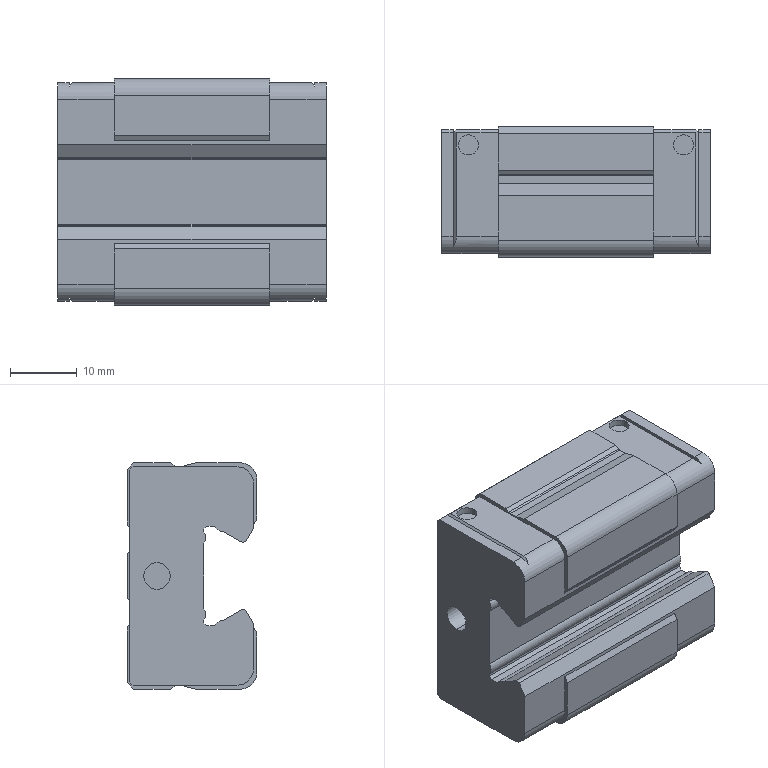Part | SolidWorks | features BaseBody 1 | 1 solid | 123 faces | box 40.3 x 19.5 x 34 mm | volume 21226 mm3 | plane 84 | cylinder 31 | cone 8 | commonest cylinder face diameters 3 x8 5 x6 2.9 x4 3.242 x4 4 x4 1.4 x3